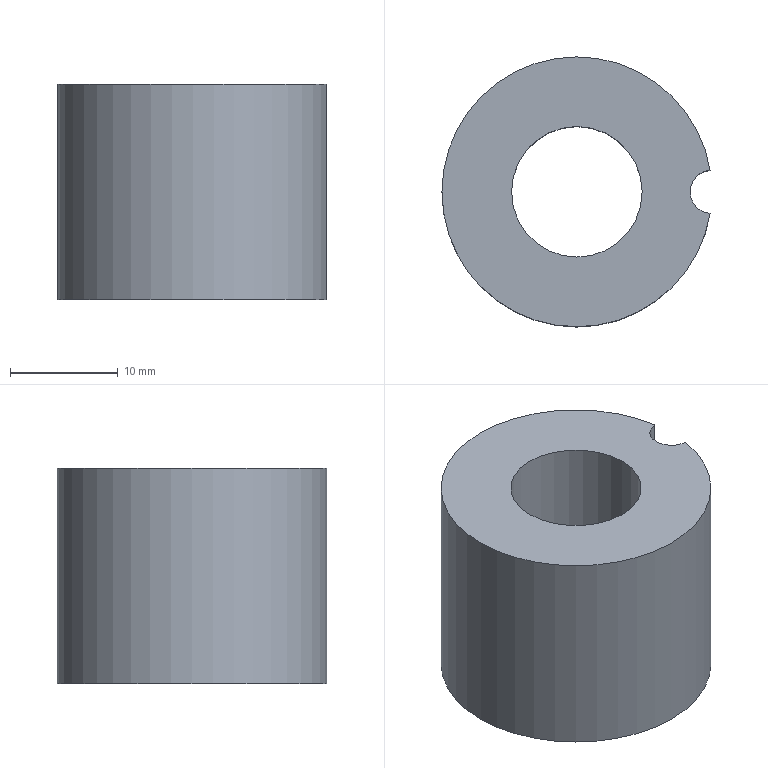Part | NX | features solid 2 | 1 solid | 7 faces | box 24.84 x 25 x 20 mm | volume 6686 mm3 | cylinder 4 | plane 3 | commonest cylinder face diameters 4 x1 12.1 x1 16.6 x1 25 x1
STEP:
#1=CARTESIAN_POINT('',(1503.836,636.771,-37.));
#2=VERTEX_POINT('',#1);
#3=CARTESIAN_POINT('',(1503.836,636.771,-17.));
#4=VERTEX_POINT('',#3);
#5=CARTESIAN_POINT('',(1503.836,636.771,-32.));
#6=DIRECTION('',(0.,0.,1.));
#7=VECTOR('',#6,1000.);
#8=LINE('',#5,#7);
#9=EDGE_CURVE('',#2,#4,#8,.T.);
#10=ORIENTED_EDGE('',*,*,#9,.F.);
#11=CARTESIAN_POINT('',(1503.836,632.784,-37.));
#12=VERTEX_POINT('',#11);
#13=CARTESIAN_POINT('',(1491.496,634.778,-37.));
#14=DIRECTION('',(0.,0.,1.));
#15=DIRECTION('',(1.,0.,0.));
#16=AXIS2_PLACEMENT_3D('',#13,#14,#15);
#17=CIRCLE('',#16,12.5);
#18=EDGE_CURVE('',#2,#12,#17,.T.);
#19=ORIENTED_EDGE('',*,*,#18,.T.);
#20=CARTESIAN_POINT('',(1503.836,632.784,-17.));
#21=VERTEX_POINT('',#20);
#22=CARTESIAN_POINT('',(1503.836,632.784,-32.));
#23=DIRECTION('',(0.,0.,1.));
#24=VECTOR('',#23,1000.);
#25=LINE('',#22,#24);
#26=EDGE_CURVE('',#21,#12,#25,.F.);
#27=ORIENTED_EDGE('',*,*,#26,.F.);
#28=CARTESIAN_POINT('',(1491.496,634.778,-17.));
#29=DIRECTION('',(0.,0.,1.));
#30=DIRECTION('',(1.,0.,0.));
#31=AXIS2_PLACEMENT_3D('',#28,#29,#30);
#32=CIRCLE('',#31,12.5);
#33=EDGE_CURVE('',#4,#21,#32,.T.);
#34=ORIENTED_EDGE('',*,*,#33,.F.);
#35=EDGE_LOOP('',(#10,#19,#27,#34));
#36=FACE_BOUND('',#35,.T.);
#37=CARTESIAN_POINT('',(1491.496,634.778,-42.));
#38=DIRECTION('',(0.,0.,1.));
#39=DIRECTION('',(1.,0.,0.));
#40=AXIS2_PLACEMENT_3D('',#37,#38,#39);
#41=CYLINDRICAL_SURFACE('',#40,12.5);
#42=ADVANCED_FACE('',(#36),#41,.T.);
#43=CARTESIAN_POINT('',(1499.796,634.778,-37.));
#44=VERTEX_POINT('',#43);
#45=CARTESIAN_POINT('',(1491.496,634.778,-37.));
#46=DIRECTION('',(0.,0.,1.));
#47=DIRECTION('',(1.,0.,0.));
#48=AXIS2_PLACEMENT_3D('',#45,#46,#47);
#49=CIRCLE('',#48,8.3);
#50=EDGE_CURVE('',#44,#44,#49,.T.);
#51=ORIENTED_EDGE('',*,*,#50,.T.);
#52=EDGE_LOOP('',(#51));
#53=FACE_BOUND('',#52,.T.);
#54=ORIENTED_EDGE('',*,*,#18,.F.);
#55=CARTESIAN_POINT('',(1503.996,634.778,-37.));
#56=DIRECTION('',(0.,0.,1.));
#57=DIRECTION('',(1.,0.,0.));
#58=AXIS2_PLACEMENT_3D('',#55,#56,#57);
#59=CIRCLE('',#58,2.);
#60=EDGE_CURVE('',#2,#12,#59,.T.);
#61=ORIENTED_EDGE('',*,*,#60,.T.);
#62=EDGE_LOOP('',(#54,#61));
#63=FACE_BOUND('',#62,.T.);
#64=CARTESIAN_POINT('',(1491.496,634.778,-37.));
#65=DIRECTION('',(0.,0.,1.));
#66=DIRECTION('',(1.,0.,0.));
#67=AXIS2_PLACEMENT_3D('',#64,#65,#66);
#68=PLANE('',#67);
#69=ADVANCED_FACE('',(#53,#63),#68,.F.);
#70=CARTESIAN_POINT('',(1497.546,634.778,-17.));
#71=VERTEX_POINT('',#70);
#72=CARTESIAN_POINT('',(1491.496,634.778,-17.));
#73=DIRECTION('',(0.,0.,1.));
#74=DIRECTION('',(1.,0.,0.));
#75=AXIS2_PLACEMENT_3D('',#72,#73,#74);
#76=CIRCLE('',#75,6.05);
#77=EDGE_CURVE('',#71,#71,#76,.T.);
#78=ORIENTED_EDGE('',*,*,#77,.F.);
#79=EDGE_LOOP('',(#78));
#80=FACE_BOUND('',#79,.T.);
#81=CARTESIAN_POINT('',(1503.996,634.778,-17.));
#82=DIRECTION('',(0.,0.,1.));
#83=DIRECTION('',(1.,0.,0.));
#84=AXIS2_PLACEMENT_3D('',#81,#82,#83);
#85=CIRCLE('',#84,2.);
#86=EDGE_CURVE('',#4,#21,#85,.T.);
#87=ORIENTED_EDGE('',*,*,#86,.F.);
#88=ORIENTED_EDGE('',*,*,#33,.T.);
#89=EDGE_LOOP('',(#87,#88));
#90=FACE_BOUND('',#89,.T.);
#91=CARTESIAN_POINT('',(1491.496,634.778,-17.));
#92=DIRECTION('',(0.,0.,1.));
#93=DIRECTION('',(1.,0.,0.));
#94=AXIS2_PLACEMENT_3D('',#91,#92,#93);
#95=PLANE('',#94);
#96=ADVANCED_FACE('',(#80,#90),#95,.T.);
#97=ORIENTED_EDGE('',*,*,#50,.F.);
#98=EDGE_LOOP('',(#97));
#99=FACE_BOUND('',#98,.T.);
#100=CARTESIAN_POINT('',(1499.796,634.778,-30.));
#101=VERTEX_POINT('',#100);
#102=CARTESIAN_POINT('',(1491.496,634.778,-30.));
#103=DIRECTION('',(0.,0.,1.));
#104=DIRECTION('',(1.,0.,0.));
#105=AXIS2_PLACEMENT_3D('',#102,#103,#104);
#106=CIRCLE('',#105,8.3);
#107=EDGE_CURVE('',#101,#101,#106,.T.);
#108=ORIENTED_EDGE('',*,*,#107,.T.);
#109=EDGE_LOOP('',(#108));
#110=FACE_BOUND('',#109,.T.);
#111=CARTESIAN_POINT('',(1491.496,634.778,-42.));
#112=DIRECTION('',(0.,0.,1.));
#113=DIRECTION('',(1.,0.,0.));
#114=AXIS2_PLACEMENT_3D('',#111,#112,#113);
#115=CYLINDRICAL_SURFACE('',#114,8.3);
#116=ADVANCED_FACE('',(#99,#110),#115,.F.);
#117=CARTESIAN_POINT('',(1497.546,634.778,-30.));
#118=VERTEX_POINT('',#117);
#119=CARTESIAN_POINT('',(1491.496,634.778,-30.));
#120=DIRECTION('',(0.,0.,1.));
#121=DIRECTION('',(1.,0.,0.));
#122=AXIS2_PLACEMENT_3D('',#119,#120,#121);
#123=CIRCLE('',#122,6.05);
#124=EDGE_CURVE('',#118,#118,#123,.T.);
#125=ORIENTED_EDGE('',*,*,#124,.T.);
#126=EDGE_LOOP('',(#125));
#127=FACE_BOUND('',#126,.T.);
#128=ORIENTED_EDGE('',*,*,#107,.F.);
#129=EDGE_LOOP('',(#128));
#130=FACE_BOUND('',#129,.T.);
#131=CARTESIAN_POINT('',(1491.496,634.778,-30.));
#132=DIRECTION('',(0.,0.,1.));
#133=DIRECTION('',(1.,0.,0.));
#134=AXIS2_PLACEMENT_3D('',#131,#132,#133);
#135=PLANE('',#134);
#136=ADVANCED_FACE('',(#127,#130),#135,.F.);
#137=ORIENTED_EDGE('',*,*,#9,.T.);
#138=ORIENTED_EDGE('',*,*,#86,.T.);
#139=ORIENTED_EDGE('',*,*,#26,.T.);
#140=ORIENTED_EDGE('',*,*,#60,.F.);
#141=EDGE_LOOP('',(#137,#138,#139,#140));
#142=FACE_BOUND('',#141,.T.);
#143=CARTESIAN_POINT('',(1503.996,634.778,-42.));
#144=DIRECTION('',(0.,0.,1.));
#145=DIRECTION('',(1.,0.,0.));
#146=AXIS2_PLACEMENT_3D('',#143,#144,#145);
#147=CYLINDRICAL_SURFACE('',#146,2.);
#148=ADVANCED_FACE('',(#142),#147,.F.);
#149=ORIENTED_EDGE('',*,*,#77,.T.);
#150=EDGE_LOOP('',(#149));
#151=FACE_BOUND('',#150,.T.);
#152=ORIENTED_EDGE('',*,*,#124,.F.);
#153=EDGE_LOOP('',(#152));
#154=FACE_BOUND('',#153,.T.);
#155=CARTESIAN_POINT('',(1491.496,634.778,-42.));
#156=DIRECTION('',(0.,0.,1.));
#157=DIRECTION('',(1.,0.,0.));
#158=AXIS2_PLACEMENT_3D('',#155,#156,#157);
#159=CYLINDRICAL_SURFACE('',#158,6.05);
#160=ADVANCED_FACE('',(#151,#154),#159,.F.);
#161=CLOSED_SHELL('',(#42,#69,#96,#116,#136,#148,#160));
#162=MANIFOLD_SOLID_BREP('',#161);
#163=(LENGTH_UNIT()NAMED_UNIT(*)SI_UNIT(.MILLI.,.METRE.));
#164=UNCERTAINTY_MEASURE_WITH_UNIT(LENGTH_MEASURE(0.00001),#163,'','');
#165=(NAMED_UNIT(*)PLANE_ANGLE_UNIT()SI_UNIT($,.RADIAN.));
#166=(NAMED_UNIT(*)SI_UNIT($,.STERADIAN.)SOLID_ANGLE_UNIT());
#167=(GEOMETRIC_REPRESENTATION_CONTEXT(3)GLOBAL_UNCERTAINTY_ASSIGNED_CONTEXT((#164))GLOBAL_UNIT_ASSIGNED_CONTEXT((#163,#165,#166))REPRESENTATION_CONTEXT('',''));
#168=ADVANCED_BREP_SHAPE_REPRESENTATION('',(#162),#167);